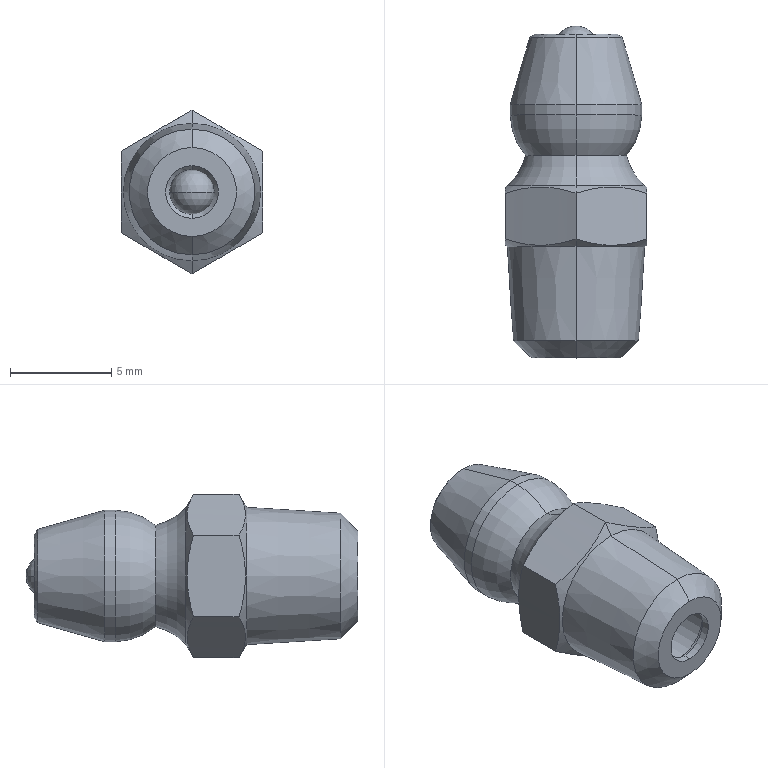Part | SolidWorks | features BaseBody 1 | 1 solid | 40 faces | box 7.001 x 16.4 x 8.083 mm | volume 360.824 mm3 | cone 14 | cylinder 8 | plane 8 | torus 6 | sphere 4 | commonest cylinder face diameters 2 x2 2.6 x2 3.4 x2 6.5 x2
STEP:
#1=CARTESIAN_POINT('',(0.,10.243,-1.007));
#2=VERTEX_POINT('',#1);
#3=CARTESIAN_POINT('',(1.007,10.243,0.));
#4=VERTEX_POINT('',#3);
#5=CARTESIAN_POINT('',(0.,10.243,0.));
#6=DIRECTION('',(0.,-1.,0.));
#7=DIRECTION('',(0.,0.,-1.));
#8=AXIS2_PLACEMENT_3D('',#5,#6,#7);
#9=CIRCLE('',#8,1.007);
#10=EDGE_CURVE('',#2,#4,#9,.T.);
#11=ORIENTED_EDGE('',*,*,#10,.T.);
#12=CARTESIAN_POINT('',(0.,8.7,0.));
#13=VERTEX_POINT('',#12);
#14=CARTESIAN_POINT('',(0.,9.8,0.));
#15=DIRECTION('',(0.,0.,-1.));
#16=DIRECTION('',(-1.,0.,0.));
#17=AXIS2_PLACEMENT_3D('',#14,#15,#16);
#18=CIRCLE('',#17,1.1);
#19=EDGE_CURVE('',#4,#13,#18,.T.);
#20=ORIENTED_EDGE('',*,*,#19,.T.);
#21=CARTESIAN_POINT('',(-1.007,10.243,0.));
#22=VERTEX_POINT('',#21);
#23=CARTESIAN_POINT('',(0.,9.8,0.));
#24=DIRECTION('',(0.,0.,1.));
#25=DIRECTION('',(1.,0.,0.));
#26=AXIS2_PLACEMENT_3D('',#23,#24,#25);
#27=CIRCLE('',#26,1.1);
#28=EDGE_CURVE('',#22,#13,#27,.T.);
#29=ORIENTED_EDGE('',*,*,#28,.F.);
#30=CARTESIAN_POINT('',(0.,10.243,0.));
#31=DIRECTION('',(0.,-1.,0.));
#32=DIRECTION('',(0.,0.,-1.));
#33=AXIS2_PLACEMENT_3D('',#30,#31,#32);
#34=CIRCLE('',#33,1.007);
#35=EDGE_CURVE('',#22,#2,#34,.T.);
#36=ORIENTED_EDGE('',*,*,#35,.T.);
#37=EDGE_LOOP('',(#11,#20,#29,#36));
#38=FACE_OUTER_BOUND('',#37,.T.);
#39=CARTESIAN_POINT('',(0.,9.8,0.));
#40=DIRECTION('',(0.,0.,-1.));
#41=DIRECTION('',(-1.,0.,0.));
#42=AXIS2_PLACEMENT_3D('',#39,#40,#41);
#43=SPHERICAL_SURFACE('',#42,1.1);
#44=ADVANCED_FACE('',(#38),#43,.T.);
#45=CARTESIAN_POINT('',(0.,10.243,1.007));
#46=VERTEX_POINT('',#45);
#47=CARTESIAN_POINT('',(0.,10.243,0.));
#48=DIRECTION('',(0.,-1.,0.));
#49=DIRECTION('',(0.,0.,-1.));
#50=AXIS2_PLACEMENT_3D('',#47,#48,#49);
#51=CIRCLE('',#50,1.007);
#52=EDGE_CURVE('',#46,#22,#51,.T.);
#53=ORIENTED_EDGE('',*,*,#52,.F.);
#54=CARTESIAN_POINT('',(0.,9.55,1.7));
#55=VERTEX_POINT('',#54);
#56=CARTESIAN_POINT('',(0.,9.55,1.7));
#57=DIRECTION('',(0.,-0.7071,0.7071));
#58=VECTOR('',#57,1000.);
#59=LINE('',#56,#58);
#60=EDGE_CURVE('',#46,#55,#59,.T.);
#61=ORIENTED_EDGE('',*,*,#60,.T.);
#62=CARTESIAN_POINT('',(0.,9.55,-1.7));
#63=VERTEX_POINT('',#62);
#64=CARTESIAN_POINT('',(0.,9.55,0.));
#65=DIRECTION('',(0.,-1.,0.));
#66=DIRECTION('',(0.,0.,-1.));
#67=AXIS2_PLACEMENT_3D('',#64,#65,#66);
#68=CIRCLE('',#67,1.7);
#69=EDGE_CURVE('',#55,#63,#68,.T.);
#70=ORIENTED_EDGE('',*,*,#69,.T.);
#71=CARTESIAN_POINT('',(0.,9.55,-1.7));
#72=DIRECTION('',(0.,-0.7071,-0.7071));
#73=VECTOR('',#72,1000.);
#74=LINE('',#71,#73);
#75=EDGE_CURVE('',#2,#63,#74,.T.);
#76=ORIENTED_EDGE('',*,*,#75,.F.);
#77=ORIENTED_EDGE('',*,*,#35,.F.);
#78=EDGE_LOOP('',(#53,#61,#70,#76,#77));
#79=FACE_OUTER_BOUND('',#78,.T.);
#80=CARTESIAN_POINT('',(0.,9.55,0.));
#81=DIRECTION('',(0.,-1.,0.));
#82=DIRECTION('',(0.,0.,-1.));
#83=AXIS2_PLACEMENT_3D('',#80,#81,#82);
#84=CONICAL_SURFACE('',#83,1.7,0.7854);
#85=ADVANCED_FACE('',(#79),#84,.F.);
#86=ORIENTED_EDGE('',*,*,#69,.F.);
#87=CARTESIAN_POINT('',(0.,-4.7,1.7));
#88=VERTEX_POINT('',#87);
#89=CARTESIAN_POINT('',(0.,-5.5,1.7));
#90=DIRECTION('',(0.,-1.,0.));
#91=VECTOR('',#90,1000.);
#92=LINE('',#89,#91);
#93=EDGE_CURVE('',#55,#88,#92,.T.);
#94=ORIENTED_EDGE('',*,*,#93,.T.);
#95=CARTESIAN_POINT('',(0.,-4.7,-1.7));
#96=VERTEX_POINT('',#95);
#97=CARTESIAN_POINT('',(0.,-4.7,0.));
#98=DIRECTION('',(0.,-1.,0.));
#99=DIRECTION('',(0.,0.,-1.));
#100=AXIS2_PLACEMENT_3D('',#97,#98,#99);
#101=CIRCLE('',#100,1.7);
#102=EDGE_CURVE('',#88,#96,#101,.T.);
#103=ORIENTED_EDGE('',*,*,#102,.T.);
#104=CARTESIAN_POINT('',(0.,-5.5,-1.7));
#105=DIRECTION('',(0.,-1.,0.));
#106=VECTOR('',#105,1000.);
#107=LINE('',#104,#106);
#108=EDGE_CURVE('',#63,#96,#107,.T.);
#109=ORIENTED_EDGE('',*,*,#108,.F.);
#110=EDGE_LOOP('',(#86,#94,#103,#109));
#111=FACE_OUTER_BOUND('',#110,.T.);
#112=CARTESIAN_POINT('',(0.,-5.5,0.));
#113=DIRECTION('',(0.,-1.,0.));
#114=DIRECTION('',(0.,0.,-1.));
#115=AXIS2_PLACEMENT_3D('',#112,#113,#114);
#116=CYLINDRICAL_SURFACE('',#115,1.7);
#117=ADVANCED_FACE('',(#111),#116,.F.);
#118=ORIENTED_EDGE('',*,*,#102,.F.);
#119=CARTESIAN_POINT('',(0.,-5.1,1.3));
#120=VERTEX_POINT('',#119);
#121=CARTESIAN_POINT('',(0.,-4.7,1.3));
#122=DIRECTION('',(1.,0.,0.));
#123=DIRECTION('',(0.,0.,-1.));
#124=AXIS2_PLACEMENT_3D('',#121,#122,#123);
#125=CIRCLE('',#124,0.4);
#126=EDGE_CURVE('',#88,#120,#125,.T.);
#127=ORIENTED_EDGE('',*,*,#126,.T.);
#128=CARTESIAN_POINT('',(0.,-5.1,-1.3));
#129=VERTEX_POINT('',#128);
#130=CARTESIAN_POINT('',(0.,-5.1,0.));
#131=DIRECTION('',(0.,-1.,0.));
#132=DIRECTION('',(0.,0.,-1.));
#133=AXIS2_PLACEMENT_3D('',#130,#131,#132);
#134=CIRCLE('',#133,1.3);
#135=EDGE_CURVE('',#120,#129,#134,.T.);
#136=ORIENTED_EDGE('',*,*,#135,.T.);
#137=CARTESIAN_POINT('',(0.,-4.7,-1.3));
#138=DIRECTION('',(-1.,0.,0.));
#139=DIRECTION('',(0.,0.,1.));
#140=AXIS2_PLACEMENT_3D('',#137,#138,#139);
#141=CIRCLE('',#140,0.4);
#142=EDGE_CURVE('',#96,#129,#141,.T.);
#143=ORIENTED_EDGE('',*,*,#142,.F.);
#144=EDGE_LOOP('',(#118,#127,#136,#143));
#145=FACE_OUTER_BOUND('',#144,.T.);
#146=CARTESIAN_POINT('',(0.,-4.7,0.));
#147=DIRECTION('',(0.,-1.,0.));
#148=DIRECTION('',(0.,0.,-1.));
#149=AXIS2_PLACEMENT_3D('',#146,#147,#148);
#150=TOROIDAL_SURFACE('',#149,1.3,0.4);
#151=ADVANCED_FACE('',(#145),#150,.F.);
#152=ORIENTED_EDGE('',*,*,#135,.F.);
#153=CARTESIAN_POINT('',(0.,-5.5,1.3));
#154=VERTEX_POINT('',#153);
#155=CARTESIAN_POINT('',(0.,-5.5,1.3));
#156=DIRECTION('',(0.,-1.,0.));
#157=VECTOR('',#156,1000.);
#158=LINE('',#155,#157);
#159=EDGE_CURVE('',#120,#154,#158,.T.);
#160=ORIENTED_EDGE('',*,*,#159,.T.);
#161=CARTESIAN_POINT('',(0.,-5.5,-1.3));
#162=VERTEX_POINT('',#161);
#163=CARTESIAN_POINT('',(0.,-5.5,0.));
#164=DIRECTION('',(0.,-1.,0.));
#165=DIRECTION('',(0.,0.,-1.));
#166=AXIS2_PLACEMENT_3D('',#163,#164,#165);
#167=CIRCLE('',#166,1.3);
#168=EDGE_CURVE('',#154,#162,#167,.T.);
#169=ORIENTED_EDGE('',*,*,#168,.T.);
#170=CARTESIAN_POINT('',(0.,-5.5,-1.3));
#171=DIRECTION('',(0.,-1.,0.));
#172=VECTOR('',#171,1000.);
#173=LINE('',#170,#172);
#174=EDGE_CURVE('',#129,#162,#173,.T.);
#175=ORIENTED_EDGE('',*,*,#174,.F.);
#176=EDGE_LOOP('',(#152,#160,#169,#175));
#177=FACE_OUTER_BOUND('',#176,.T.);
#178=CARTESIAN_POINT('',(0.,-5.5,0.));
#179=DIRECTION('',(0.,-1.,0.));
#180=DIRECTION('',(0.,0.,-1.));
#181=AXIS2_PLACEMENT_3D('',#178,#179,#180);
#182=CYLINDRICAL_SURFACE('',#181,1.3);
#183=ADVANCED_FACE('',(#177),#182,.F.);
#184=CARTESIAN_POINT('',(0.,-5.5,-2.2));
#185=VERTEX_POINT('',#184);
#186=CARTESIAN_POINT('',(0.,-5.5,2.2));
#187=VERTEX_POINT('',#186);
#188=CARTESIAN_POINT('',(0.,-5.5,0.));
#189=DIRECTION('',(0.,-1.,0.));
#190=DIRECTION('',(0.,0.,-1.));
#191=AXIS2_PLACEMENT_3D('',#188,#189,#190);
#192=CIRCLE('',#191,2.2);
#193=EDGE_CURVE('',#185,#187,#192,.T.);
#194=ORIENTED_EDGE('',*,*,#193,.F.);
#195=CARTESIAN_POINT('',(0.,-4.652,-3.103));
#196=VERTEX_POINT('',#195);
#197=CARTESIAN_POINT('',(0.,-4.652,-3.103));
#198=DIRECTION('',(0.,0.6847,-0.7288));
#199=VECTOR('',#198,1000.);
#200=LINE('',#197,#199);
#201=EDGE_CURVE('',#185,#196,#200,.T.);
#202=ORIENTED_EDGE('',*,*,#201,.T.);
#203=CARTESIAN_POINT('',(0.,-4.652,3.103));
#204=VERTEX_POINT('',#203);
#205=CARTESIAN_POINT('',(0.,-4.652,0.));
#206=DIRECTION('',(0.,-1.,0.));
#207=DIRECTION('',(0.,0.,-1.));
#208=AXIS2_PLACEMENT_3D('',#205,#206,#207);
#209=CIRCLE('',#208,3.103);
#210=EDGE_CURVE('',#196,#204,#209,.T.);
#211=ORIENTED_EDGE('',*,*,#210,.T.);
#212=CARTESIAN_POINT('',(0.,-4.652,3.103));
#213=DIRECTION('',(0.,0.6847,0.7288));
#214=VECTOR('',#213,1000.);
#215=LINE('',#212,#214);
#216=EDGE_CURVE('',#187,#204,#215,.T.);
#217=ORIENTED_EDGE('',*,*,#216,.F.);
#218=EDGE_LOOP('',(#194,#202,#211,#217));
#219=FACE_OUTER_BOUND('',#218,.T.);
#220=CARTESIAN_POINT('',(0.,-4.652,0.));
#221=DIRECTION('',(0.,1.,0.));
#222=DIRECTION('',(0.,0.,1.));
#223=AXIS2_PLACEMENT_3D('',#220,#221,#222);
#224=CONICAL_SURFACE('',#223,3.103,0.8166);
#225=ADVANCED_FACE('',(#219),#224,.T.);
#226=ORIENTED_EDGE('',*,*,#210,.F.);
#227=CARTESIAN_POINT('',(0.,0.,-3.394));
#228=VERTEX_POINT('',#227);
#229=CARTESIAN_POINT('',(0.,0.,-3.394));
#230=DIRECTION('',(0.,0.998,-0.06244));
#231=VECTOR('',#230,1000.);
#232=LINE('',#229,#231);
#233=EDGE_CURVE('',#196,#228,#232,.T.);
#234=ORIENTED_EDGE('',*,*,#233,.T.);
#235=CARTESIAN_POINT('',(0.,0.,3.394));
#236=VERTEX_POINT('',#235);
#237=CARTESIAN_POINT('',(0.,0.,0.));
#238=DIRECTION('',(0.,-1.,0.));
#239=DIRECTION('',(0.,0.,-1.));
#240=AXIS2_PLACEMENT_3D('',#237,#238,#239);
#241=CIRCLE('',#240,3.394);
#242=EDGE_CURVE('',#228,#236,#241,.T.);
#243=ORIENTED_EDGE('',*,*,#242,.T.);
#244=CARTESIAN_POINT('',(0.,0.,3.394));
#245=DIRECTION('',(0.,0.998,0.06244));
#246=VECTOR('',#245,1000.);
#247=LINE('',#244,#246);
#248=EDGE_CURVE('',#204,#236,#247,.T.);
#249=ORIENTED_EDGE('',*,*,#248,.F.);
#250=EDGE_LOOP('',(#226,#234,#243,#249));
#251=FACE_OUTER_BOUND('',#250,.T.);
#252=CARTESIAN_POINT('',(0.,0.,0.));
#253=DIRECTION('',(0.,1.,0.));
#254=DIRECTION('',(0.,0.,1.));
#255=AXIS2_PLACEMENT_3D('',#252,#253,#254);
#256=CONICAL_SURFACE('',#255,3.394,0.06248);
#257=ADVANCED_FACE('',(#251),#256,.T.);
#258=ORIENTED_EDGE('',*,*,#242,.F.);
#259=CARTESIAN_POINT('',(0.,0.374,-4.041));
#260=VERTEX_POINT('',#259);
#261=CARTESIAN_POINT('',(0.,1.216,-5.5));
#262=DIRECTION('',(0.,0.5,-0.866));
#263=VECTOR('',#262,1000.);
#264=LINE('',#261,#263);
#265=EDGE_CURVE('',#228,#260,#264,.T.);
#266=ORIENTED_EDGE('',*,*,#265,.T.);
#267=CARTESIAN_POINT('',(3.5,0.374,-2.021));
#268=VERTEX_POINT('',#267);
#269=CARTESIAN_POINT('',(0.,0.374,-4.041));
#270=CARTESIAN_POINT('',(0.1588,0.321,-3.95));
#271=CARTESIAN_POINT('',(0.303,0.2771,-3.865));
#272=CARTESIAN_POINT('',(0.585,0.2025,-3.702));
#273=CARTESIAN_POINT('',(0.7229,0.1719,-3.623));
#274=CARTESIAN_POINT('',(1.15,0.09295,-3.378));
#275=CARTESIAN_POINT('',(1.457,0.0621,-3.201));
#276=CARTESIAN_POINT('',(1.896,0.0612,-2.946));
#277=CARTESIAN_POINT('',(2.041,0.0685,-2.864));
#278=CARTESIAN_POINT('',(2.338,0.09717,-2.693));
#279=CARTESIAN_POINT('',(2.488,0.1184,-2.606));
#280=CARTESIAN_POINT('',(2.78,0.1726,-2.436));
#281=CARTESIAN_POINT('',(2.918,0.2041,-2.355));
#282=CARTESIAN_POINT('',(3.199,0.2783,-2.193));
#283=CARTESIAN_POINT('',(3.343,0.3216,-2.111));
#284=CARTESIAN_POINT('',(3.5,0.374,-2.021));
#285=B_SPLINE_CURVE_WITH_KNOTS('',3,(#269,#270,#271,#272,#273,#274,#275,#276,#277,#278,#279,#280,#281,#282,#283,#284),.UNSPECIFIED.,.F.,.F.,(4,2,2,2,2,2,2,4),(0.0002381,0.5104,1.021,2.041,2.551,3.061,3.572,4.082),.UNSPECIFIED.);
#286=EDGE_CURVE('',#260,#268,#285,.T.);
#287=ORIENTED_EDGE('',*,*,#286,.T.);
#288=CARTESIAN_POINT('',(3.5,0.374,2.021));
#289=VERTEX_POINT('',#288);
#290=CARTESIAN_POINT('',(3.5,0.374,-2.021));
#291=CARTESIAN_POINT('',(3.5,0.3259,-1.854));
#292=CARTESIAN_POINT('',(3.5,0.2835,-1.693));
#293=CARTESIAN_POINT('',(3.5,0.2061,-1.357));
#294=CARTESIAN_POINT('',(3.5,0.1735,-1.194));
#295=CARTESIAN_POINT('',(3.5,0.1183,-0.8526));
#296=CARTESIAN_POINT('',(3.501,0.09717,-0.6799));
#297=CARTESIAN_POINT('',(3.501,0.06865,-0.337));
#298=CARTESIAN_POINT('',(3.5,0.06131,-0.1677));
#299=CARTESIAN_POINT('',(3.5,0.06147,0.3344));
#300=CARTESIAN_POINT('',(3.5,0.09108,0.6846));
#301=CARTESIAN_POINT('',(3.5,0.1735,1.194));
#302=CARTESIAN_POINT('',(3.5,0.2062,1.357));
#303=CARTESIAN_POINT('',(3.5,0.2835,1.693));
#304=CARTESIAN_POINT('',(3.5,0.3263,1.856));
#305=CARTESIAN_POINT('',(3.5,0.374,2.021));
#306=B_SPLINE_CURVE_WITH_KNOTS('',3,(#290,#291,#292,#293,#294,#295,#296,#297,#298,#299,#300,#301,#302,#303,#304,#305),.UNSPECIFIED.,.F.,.F.,(4,2,2,2,2,2,2,4),(4.59,5.104,5.618,6.132,6.646,7.674,8.188,8.702),.UNSPECIFIED.);
#307=EDGE_CURVE('',#268,#289,#306,.T.);
#308=ORIENTED_EDGE('',*,*,#307,.T.);
#309=CARTESIAN_POINT('',(0.,0.374,4.041));
#310=VERTEX_POINT('',#309);
#311=CARTESIAN_POINT('',(3.5,0.374,2.021));
#312=CARTESIAN_POINT('',(3.341,0.321,2.112));
#313=CARTESIAN_POINT('',(3.195,0.2771,2.195));
#314=CARTESIAN_POINT('',(2.913,0.2025,2.357));
#315=CARTESIAN_POINT('',(2.777,0.1719,2.438));
#316=CARTESIAN_POINT('',(2.35,0.09295,2.685));
#317=CARTESIAN_POINT('',(2.044,0.0621,2.863));
#318=CARTESIAN_POINT('',(1.604,0.0612,3.115));
#319=CARTESIAN_POINT('',(1.46,0.0685,3.199));
#320=CARTESIAN_POINT('',(1.163,0.09717,3.371));
#321=CARTESIAN_POINT('',(1.013,0.1184,3.457));
#322=CARTESIAN_POINT('',(0.7202,0.1726,3.625));
#323=CARTESIAN_POINT('',(0.5806,0.2041,3.705));
#324=CARTESIAN_POINT('',(0.2992,0.2783,3.867));
#325=CARTESIAN_POINT('',(0.1571,0.3216,3.951));
#326=CARTESIAN_POINT('',(0.,0.374,4.041));
#327=B_SPLINE_CURVE_WITH_KNOTS('',3,(#311,#312,#313,#314,#315,#316,#317,#318,#319,#320,#321,#322,#323,#324,#325,#326),.UNSPECIFIED.,.F.,.F.,(4,2,2,2,2,2,2,4),(0.0002381,0.5104,1.021,2.041,2.551,3.061,3.572,4.082),.UNSPECIFIED.);
#328=EDGE_CURVE('',#289,#310,#327,.T.);
#329=ORIENTED_EDGE('',*,*,#328,.T.);
#330=CARTESIAN_POINT('',(0.,1.216,5.5));
#331=DIRECTION('',(0.,0.5,0.866));
#332=VECTOR('',#331,1000.);
#333=LINE('',#330,#332);
#334=EDGE_CURVE('',#236,#310,#333,.T.);
#335=ORIENTED_EDGE('',*,*,#334,.F.);
#336=EDGE_LOOP('',(#258,#266,#287,#308,#329,#335));
#337=FACE_OUTER_BOUND('',#336,.T.);
#338=CARTESIAN_POINT('',(0.,1.216,0.));
#339=DIRECTION('',(0.,1.,0.));
#340=DIRECTION('',(0.,0.,1.));
#341=AXIS2_PLACEMENT_3D('',#338,#339,#340);
#342=CONICAL_SURFACE('',#341,5.5,1.047);
#343=ADVANCED_FACE('',(#337),#342,.T.);
#344=CARTESIAN_POINT('',(0.,3.,-3.394));
#345=VERTEX_POINT('',#344);
#346=CARTESIAN_POINT('',(0.,3.,3.394));
#347=VERTEX_POINT('',#346);
#348=CARTESIAN_POINT('',(0.,3.,0.));
#349=DIRECTION('',(0.,-1.,0.));
#350=DIRECTION('',(0.,0.,-1.));
#351=AXIS2_PLACEMENT_3D('',#348,#349,#350);
#352=CIRCLE('',#351,3.394);
#353=EDGE_CURVE('',#345,#347,#352,.T.);
#354=ORIENTED_EDGE('',*,*,#353,.T.);
#355=CARTESIAN_POINT('',(0.,2.626,4.041));
#356=VERTEX_POINT('',#355);
#357=CARTESIAN_POINT('',(0.,3.,3.394));
#358=DIRECTION('',(0.,-0.5,0.866));
#359=VECTOR('',#358,1000.);
#360=LINE('',#357,#359);
#361=EDGE_CURVE('',#347,#356,#360,.T.);
#362=ORIENTED_EDGE('',*,*,#361,.T.);
#363=CARTESIAN_POINT('',(3.5,2.626,2.021));
#364=VERTEX_POINT('',#363);
#365=CARTESIAN_POINT('',(0.,2.626,4.041));
#366=CARTESIAN_POINT('',(0.1588,2.679,3.95));
#367=CARTESIAN_POINT('',(0.303,2.723,3.865));
#368=CARTESIAN_POINT('',(0.585,2.797,3.702));
#369=CARTESIAN_POINT('',(0.7229,2.828,3.623));
#370=CARTESIAN_POINT('',(1.15,2.907,3.378));
#371=CARTESIAN_POINT('',(1.457,2.938,3.201));
#372=CARTESIAN_POINT('',(1.896,2.939,2.946));
#373=CARTESIAN_POINT('',(2.041,2.932,2.864));
#374=CARTESIAN_POINT('',(2.338,2.903,2.693));
#375=CARTESIAN_POINT('',(2.488,2.882,2.606));
#376=CARTESIAN_POINT('',(2.78,2.827,2.436));
#377=CARTESIAN_POINT('',(2.918,2.796,2.355));
#378=CARTESIAN_POINT('',(3.199,2.722,2.193));
#379=CARTESIAN_POINT('',(3.343,2.678,2.111));
#380=CARTESIAN_POINT('',(3.5,2.626,2.021));
#381=B_SPLINE_CURVE_WITH_KNOTS('',3,(#365,#366,#367,#368,#369,#370,#371,#372,#373,#374,#375,#376,#377,#378,#379,#380),.UNSPECIFIED.,.F.,.F.,(4,2,2,2,2,2,2,4),(0.0002381,0.5104,1.021,2.041,2.551,3.061,3.572,4.082),.UNSPECIFIED.);
#382=EDGE_CURVE('',#356,#364,#381,.T.);
#383=ORIENTED_EDGE('',*,*,#382,.T.);
#384=CARTESIAN_POINT('',(3.5,2.626,-2.021));
#385=VERTEX_POINT('',#384);
#386=CARTESIAN_POINT('',(3.5,2.626,2.021));
#387=CARTESIAN_POINT('',(3.5,2.674,1.854));
#388=CARTESIAN_POINT('',(3.5,2.716,1.693));
#389=CARTESIAN_POINT('',(3.5,2.794,1.357));
#390=CARTESIAN_POINT('',(3.5,2.826,1.194));
#391=CARTESIAN_POINT('',(3.5,2.882,0.8526));
#392=CARTESIAN_POINT('',(3.501,2.903,0.6799));
#393=CARTESIAN_POINT('',(3.501,2.931,0.337));
#394=CARTESIAN_POINT('',(3.5,2.939,0.1677));
#395=CARTESIAN_POINT('',(3.5,2.939,-0.3344));
#396=CARTESIAN_POINT('',(3.5,2.909,-0.6846));
#397=CARTESIAN_POINT('',(3.5,2.826,-1.194));
#398=CARTESIAN_POINT('',(3.5,2.794,-1.357));
#399=CARTESIAN_POINT('',(3.5,2.716,-1.693));
#400=CARTESIAN_POINT('',(3.5,2.674,-1.856));
#401=CARTESIAN_POINT('',(3.5,2.626,-2.021));
#402=B_SPLINE_CURVE_WITH_KNOTS('',3,(#386,#387,#388,#389,#390,#391,#392,#393,#394,#395,#396,#397,#398,#399,#400,#401),.UNSPECIFIED.,.F.,.F.,(4,2,2,2,2,2,2,4),(4.59,5.104,5.618,6.132,6.646,7.674,8.188,8.702),.UNSPECIFIED.);
#403=EDGE_CURVE('',#364,#385,#402,.T.);
#404=ORIENTED_EDGE('',*,*,#403,.T.);
#405=CARTESIAN_POINT('',(0.,2.626,-4.041));
#406=VERTEX_POINT('',#405);
#407=CARTESIAN_POINT('',(3.5,2.626,-2.021));
#408=CARTESIAN_POINT('',(3.341,2.679,-2.112));
#409=CARTESIAN_POINT('',(3.195,2.723,-2.195));
#410=CARTESIAN_POINT('',(2.913,2.797,-2.357));
#411=CARTESIAN_POINT('',(2.777,2.828,-2.438));
#412=CARTESIAN_POINT('',(2.35,2.907,-2.685));
#413=CARTESIAN_POINT('',(2.044,2.938,-2.863));
#414=CARTESIAN_POINT('',(1.604,2.939,-3.115));
#415=CARTESIAN_POINT('',(1.46,2.932,-3.199));
#416=CARTESIAN_POINT('',(1.163,2.903,-3.371));
#417=CARTESIAN_POINT('',(1.013,2.882,-3.457));
#418=CARTESIAN_POINT('',(0.7202,2.827,-3.625));
#419=CARTESIAN_POINT('',(0.5806,2.796,-3.705));
#420=CARTESIAN_POINT('',(0.2992,2.722,-3.867));
#421=CARTESIAN_POINT('',(0.1571,2.678,-3.951));
#422=CARTESIAN_POINT('',(0.,2.626,-4.041));
#423=B_SPLINE_CURVE_WITH_KNOTS('',3,(#407,#408,#409,#410,#411,#412,#413,#414,#415,#416,#417,#418,#419,#420,#421,#422),.UNSPECIFIED.,.F.,.F.,(4,2,2,2,2,2,2,4),(0.0002381,0.5104,1.021,2.041,2.551,3.061,3.572,4.082),.UNSPECIFIED.);
#424=EDGE_CURVE('',#385,#406,#423,.T.);
#425=ORIENTED_EDGE('',*,*,#424,.T.);
#426=CARTESIAN_POINT('',(0.,3.,-3.394));
#427=DIRECTION('',(0.,-0.5,-0.866));
#428=VECTOR('',#427,1000.);
#429=LINE('',#426,#428);
#430=EDGE_CURVE('',#345,#406,#429,.T.);
#431=ORIENTED_EDGE('',*,*,#430,.F.);
#432=EDGE_LOOP('',(#354,#362,#383,#404,#425,#431));
#433=FACE_OUTER_BOUND('',#432,.T.);
#434=CARTESIAN_POINT('',(0.,3.,0.));
#435=DIRECTION('',(0.,-1.,0.));
#436=DIRECTION('',(0.,0.,-1.));
#437=AXIS2_PLACEMENT_3D('',#434,#435,#436);
#438=CONICAL_SURFACE('',#437,3.394,1.047);
#439=ADVANCED_FACE('',(#433),#438,.T.);
#440=CARTESIAN_POINT('',(0.,3.,0.));
#441=DIRECTION('',(0.,-1.,0.));
#442=DIRECTION('',(0.,0.,-1.));
#443=AXIS2_PLACEMENT_3D('',#440,#441,#442);
#444=CIRCLE('',#443,3.394);
#445=EDGE_CURVE('',#347,#345,#444,.T.);
#446=ORIENTED_EDGE('',*,*,#445,.F.);
#447=CARTESIAN_POINT('',(0.,4.5,2.5));
#448=VERTEX_POINT('',#447);
#449=CARTESIAN_POINT('',(0.,5.166,5.323));
#450=DIRECTION('',(1.,0.,0.));
#451=DIRECTION('',(0.,0.,-1.));
#452=AXIS2_PLACEMENT_3D('',#449,#450,#451);
#453=CIRCLE('',#452,2.9);
#454=EDGE_CURVE('',#347,#448,#453,.T.);
#455=ORIENTED_EDGE('',*,*,#454,.T.);
#456=CARTESIAN_POINT('',(0.,4.5,-2.5));
#457=VERTEX_POINT('',#456);
#458=CARTESIAN_POINT('',(0.,4.5,0.));
#459=DIRECTION('',(0.,-1.,0.));
#460=DIRECTION('',(0.,0.,-1.));
#461=AXIS2_PLACEMENT_3D('',#458,#459,#460);
#462=CIRCLE('',#461,2.5);
#463=EDGE_CURVE('',#448,#457,#462,.T.);
#464=ORIENTED_EDGE('',*,*,#463,.T.);
#465=CARTESIAN_POINT('',(0.,5.166,-5.323));
#466=DIRECTION('',(-1.,0.,0.));
#467=DIRECTION('',(0.,0.,1.));
#468=AXIS2_PLACEMENT_3D('',#465,#466,#467);
#469=CIRCLE('',#468,2.9);
#470=EDGE_CURVE('',#345,#457,#469,.T.);
#471=ORIENTED_EDGE('',*,*,#470,.F.);
#472=EDGE_LOOP('',(#446,#455,#464,#471));
#473=FACE_OUTER_BOUND('',#472,.T.);
#474=CARTESIAN_POINT('',(0.,5.166,0.));
#475=DIRECTION('',(0.,-1.,0.));
#476=DIRECTION('',(0.,0.,-1.));
#477=AXIS2_PLACEMENT_3D('',#474,#475,#476);
#478=TOROIDAL_SURFACE('',#477,5.323,2.9);
#479=ADVANCED_FACE('',(#473),#478,.F.);
#480=CARTESIAN_POINT('',(0.,6.5,-3.25));
#481=VERTEX_POINT('',#480);
#482=CARTESIAN_POINT('',(0.,6.5,3.25));
#483=VERTEX_POINT('',#482);
#484=CARTESIAN_POINT('',(0.,6.5,0.));
#485=DIRECTION('',(0.,-1.,0.));
#486=DIRECTION('',(0.,0.,-1.));
#487=AXIS2_PLACEMENT_3D('',#484,#485,#486);
#488=CIRCLE('',#487,3.25);
#489=EDGE_CURVE('',#481,#483,#488,.T.);
#490=ORIENTED_EDGE('',*,*,#489,.T.);
#491=CARTESIAN_POINT('',(0.,6.578,0.0009308));
#492=DIRECTION('',(1.,0.,0.));
#493=DIRECTION('',(0.,0.,-1.));
#494=AXIS2_PLACEMENT_3D('',#491,#492,#493);
#495=CIRCLE('',#494,3.25);
#496=EDGE_CURVE('',#483,#448,#495,.T.);
#497=ORIENTED_EDGE('',*,*,#496,.T.);
#498=CARTESIAN_POINT('',(0.,4.5,0.));
#499=DIRECTION('',(0.,-1.,0.));
#500=DIRECTION('',(0.,0.,-1.));
#501=AXIS2_PLACEMENT_3D('',#498,#499,#500);
#502=CIRCLE('',#501,2.5);
#503=EDGE_CURVE('',#457,#448,#502,.T.);
#504=ORIENTED_EDGE('',*,*,#503,.F.);
#505=CARTESIAN_POINT('',(0.,6.578,-0.0009308));
#506=DIRECTION('',(-1.,0.,0.));
#507=DIRECTION('',(0.,0.,1.));
#508=AXIS2_PLACEMENT_3D('',#505,#506,#507);
#509=CIRCLE('',#508,3.25);
#510=EDGE_CURVE('',#481,#457,#509,.T.);
#511=ORIENTED_EDGE('',*,*,#510,.F.);
#512=EDGE_LOOP('',(#490,#497,#504,#511));
#513=FACE_OUTER_BOUND('',#512,.T.);
#514=CARTESIAN_POINT('',(0.,6.578,0.));
#515=DIRECTION('',(0.,-1.,0.));
#516=DIRECTION('',(0.,0.,-1.));
#517=AXIS2_PLACEMENT_3D('',#514,#515,#516);
#518=TOROIDAL_SURFACE('',#517,0.0009308,3.25);
#519=ADVANCED_FACE('',(#513),#518,.T.);
#520=CARTESIAN_POINT('',(0.,7.,-3.25));
#521=VERTEX_POINT('',#520);
#522=CARTESIAN_POINT('',(0.,7.,3.25));
#523=VERTEX_POINT('',#522);
#524=CARTESIAN_POINT('',(0.,7.,0.));
#525=DIRECTION('',(0.,-1.,0.));
#526=DIRECTION('',(0.,0.,-1.));
#527=AXIS2_PLACEMENT_3D('',#524,#525,#526);
#528=CIRCLE('',#527,3.25);
#529=EDGE_CURVE('',#521,#523,#528,.T.);
#530=ORIENTED_EDGE('',*,*,#529,.T.);
#531=CARTESIAN_POINT('',(0.,-5.5,3.25));
#532=DIRECTION('',(0.,-1.,0.));
#533=VECTOR('',#532,1000.);
#534=LINE('',#531,#533);
#535=EDGE_CURVE('',#523,#483,#534,.T.);
#536=ORIENTED_EDGE('',*,*,#535,.T.);
#537=ORIENTED_EDGE('',*,*,#489,.F.);
#538=CARTESIAN_POINT('',(0.,-5.5,-3.25));
#539=DIRECTION('',(0.,-1.,0.));
#540=VECTOR('',#539,1000.);
#541=LINE('',#538,#540);
#542=EDGE_CURVE('',#521,#481,#541,.T.);
#543=ORIENTED_EDGE('',*,*,#542,.F.);
#544=EDGE_LOOP('',(#530,#536,#537,#543));
#545=FACE_OUTER_BOUND('',#544,.T.);
#546=CARTESIAN_POINT('',(0.,-5.5,0.));
#547=DIRECTION('',(0.,-1.,0.));
#548=DIRECTION('',(0.,0.,-1.));
#549=AXIS2_PLACEMENT_3D('',#546,#547,#548);
#550=CYLINDRICAL_SURFACE('',#549,3.25);
#551=ADVANCED_FACE('',(#545),#550,.T.);
#552=CARTESIAN_POINT('',(0.,10.315,-2.303));
#553=VERTEX_POINT('',#552);
#554=CARTESIAN_POINT('',(0.,10.315,2.303));
#555=VERTEX_POINT('',#554);
#556=CARTESIAN_POINT('',(0.,10.315,0.));
#557=DIRECTION('',(0.,-1.,0.));
#558=DIRECTION('',(0.,0.,-1.));
#559=AXIS2_PLACEMENT_3D('',#556,#557,#558);
#560=CIRCLE('',#559,2.303);
#561=EDGE_CURVE('',#553,#555,#560,.T.);
#562=ORIENTED_EDGE('',*,*,#561,.T.);
#563=CARTESIAN_POINT('',(0.,10.315,2.303));
#564=DIRECTION('',(0.,-0.9615,0.2748));
#565=VECTOR('',#564,1000.);
#566=LINE('',#563,#565);
#567=EDGE_CURVE('',#555,#523,#566,.T.);
#568=ORIENTED_EDGE('',*,*,#567,.T.);
#569=ORIENTED_EDGE('',*,*,#529,.F.);
#570=CARTESIAN_POINT('',(0.,10.315,-2.303));
#571=DIRECTION('',(0.,-0.9615,-0.2748));
#572=VECTOR('',#571,1000.);
#573=LINE('',#570,#572);
#574=EDGE_CURVE('',#553,#521,#573,.T.);
#575=ORIENTED_EDGE('',*,*,#574,.F.);
#576=EDGE_LOOP('',(#562,#568,#569,#575));
#577=FACE_OUTER_BOUND('',#576,.T.);
#578=CARTESIAN_POINT('',(0.,10.315,0.));
#579=DIRECTION('',(0.,-1.,0.));
#580=DIRECTION('',(0.,0.,-1.));
#581=AXIS2_PLACEMENT_3D('',#578,#579,#580);
#582=CONICAL_SURFACE('',#581,2.303,0.2784);
#583=ADVANCED_FACE('',(#577),#582,.T.);
#584=CARTESIAN_POINT('',(0.,10.5,-2.057));
#585=VERTEX_POINT('',#584);
#586=CARTESIAN_POINT('',(0.,10.5,2.057));
#587=VERTEX_POINT('',#586);
#588=CARTESIAN_POINT('',(0.,10.5,0.));
#589=DIRECTION('',(0.,-1.,0.));
#590=DIRECTION('',(0.,0.,-1.));
#591=AXIS2_PLACEMENT_3D('',#588,#589,#590);
#592=CIRCLE('',#591,2.057);
#593=EDGE_CURVE('',#585,#587,#592,.T.);
#594=ORIENTED_EDGE('',*,*,#593,.T.);
#595=CARTESIAN_POINT('',(0.,10.5,2.057));
#596=DIRECTION('',(0.,-0.6022,0.7984));
#597=VECTOR('',#596,1000.);
#598=LINE('',#595,#597);
#599=EDGE_CURVE('',#587,#555,#598,.T.);
#600=ORIENTED_EDGE('',*,*,#599,.T.);
#601=ORIENTED_EDGE('',*,*,#561,.F.);
#602=CARTESIAN_POINT('',(0.,10.5,-2.057));
#603=DIRECTION('',(0.,-0.6022,-0.7984));
#604=VECTOR('',#603,1000.);
#605=LINE('',#602,#604);
#606=EDGE_CURVE('',#585,#553,#605,.T.);
#607=ORIENTED_EDGE('',*,*,#606,.F.);
#608=EDGE_LOOP('',(#594,#600,#601,#607));
#609=FACE_OUTER_BOUND('',#608,.T.);
#610=CARTESIAN_POINT('',(0.,10.5,0.));
#611=DIRECTION('',(0.,-1.,0.));
#612=DIRECTION('',(0.,0.,-1.));
#613=AXIS2_PLACEMENT_3D('',#610,#611,#612);
#614=CONICAL_SURFACE('',#613,2.057,0.9246);
#615=ADVANCED_FACE('',(#609),#614,.T.);
#616=CARTESIAN_POINT('',(0.,10.5,1.));
#617=VERTEX_POINT('',#616);
#618=CARTESIAN_POINT('',(0.,10.5,-1.));
#619=VERTEX_POINT('',#618);
#620=CARTESIAN_POINT('',(0.,10.5,0.));
#621=DIRECTION('',(0.,-1.,0.));
#622=DIRECTION('',(0.,0.,-1.));
#623=AXIS2_PLACEMENT_3D('',#620,#621,#622);
#624=CIRCLE('',#623,1.);
#625=EDGE_CURVE('',#617,#619,#624,.T.);
#626=ORIENTED_EDGE('',*,*,#625,.F.);
#627=CARTESIAN_POINT('',(0.,10.258,1.));
#628=VERTEX_POINT('',#627);
#629=CARTESIAN_POINT('',(0.,-5.5,1.));
#630=DIRECTION('',(0.,-1.,0.));
#631=VECTOR('',#630,1000.);
#632=LINE('',#629,#631);
#633=EDGE_CURVE('',#617,#628,#632,.T.);
#634=ORIENTED_EDGE('',*,*,#633,.T.);
#635=CARTESIAN_POINT('',(-1.,10.258,0.));
#636=VERTEX_POINT('',#635);
#637=CARTESIAN_POINT('',(0.,10.258,0.));
#638=DIRECTION('',(0.,-1.,0.));
#639=DIRECTION('',(0.,0.,-1.));
#640=AXIS2_PLACEMENT_3D('',#637,#638,#639);
#641=CIRCLE('',#640,1.);
#642=EDGE_CURVE('',#628,#636,#641,.T.);
#643=ORIENTED_EDGE('',*,*,#642,.T.);
#644=CARTESIAN_POINT('',(0.,10.258,-1.));
#645=VERTEX_POINT('',#644);
#646=CARTESIAN_POINT('',(0.,10.258,0.));
#647=DIRECTION('',(0.,-1.,0.));
#648=DIRECTION('',(0.,0.,-1.));
#649=AXIS2_PLACEMENT_3D('',#646,#647,#648);
#650=CIRCLE('',#649,1.);
#651=EDGE_CURVE('',#636,#645,#650,.T.);
#652=ORIENTED_EDGE('',*,*,#651,.T.);
#653=CARTESIAN_POINT('',(0.,-5.5,-1.));
#654=DIRECTION('',(0.,-1.,0.));
#655=VECTOR('',#654,1000.);
#656=LINE('',#653,#655);
#657=EDGE_CURVE('',#619,#645,#656,.T.);
#658=ORIENTED_EDGE('',*,*,#657,.F.);
#659=EDGE_LOOP('',(#626,#634,#643,#652,#658));
#660=FACE_OUTER_BOUND('',#659,.T.);
#661=CARTESIAN_POINT('',(0.,-5.5,0.));
#662=DIRECTION('',(0.,-1.,0.));
#663=DIRECTION('',(0.,0.,-1.));
#664=AXIS2_PLACEMENT_3D('',#661,#662,#663);
#665=CYLINDRICAL_SURFACE('',#664,1.);
#666=ADVANCED_FACE('',(#660),#665,.F.);
#667=CARTESIAN_POINT('',(0.,10.9,0.));
#668=VERTEX_POINT('',#667);
#669=CARTESIAN_POINT('',(1.,10.258,0.));
#670=VERTEX_POINT('',#669);
#671=CARTESIAN_POINT('',(0.,9.8,0.));
#672=DIRECTION('',(0.,0.,-1.));
#673=DIRECTION('',(-1.,0.,0.));
#674=AXIS2_PLACEMENT_3D('',#671,#672,#673);
#675=CIRCLE('',#674,1.1);
#676=EDGE_CURVE('',#668,#670,#675,.T.);
#677=ORIENTED_EDGE('',*,*,#676,.F.);
#678=CARTESIAN_POINT('',(0.,9.8,0.));
#679=DIRECTION('',(0.,0.,1.));
#680=DIRECTION('',(1.,0.,0.));
#681=AXIS2_PLACEMENT_3D('',#678,#679,#680);
#682=CIRCLE('',#681,1.1);
#683=EDGE_CURVE('',#668,#636,#682,.T.);
#684=ORIENTED_EDGE('',*,*,#683,.T.);
#685=ORIENTED_EDGE('',*,*,#642,.F.);
#686=CARTESIAN_POINT('',(0.,10.258,0.));
#687=DIRECTION('',(0.,-1.,0.));
#688=DIRECTION('',(0.,0.,-1.));
#689=AXIS2_PLACEMENT_3D('',#686,#687,#688);
#690=CIRCLE('',#689,1.);
#691=EDGE_CURVE('',#670,#628,#690,.T.);
#692=ORIENTED_EDGE('',*,*,#691,.F.);
#693=EDGE_LOOP('',(#677,#684,#685,#692));
#694=FACE_OUTER_BOUND('',#693,.T.);
#695=CARTESIAN_POINT('',(0.,9.8,0.));
#696=DIRECTION('',(0.,0.,1.));
#697=DIRECTION('',(1.,0.,0.));
#698=AXIS2_PLACEMENT_3D('',#695,#696,#697);
#699=SPHERICAL_SURFACE('',#698,1.1);
#700=ADVANCED_FACE('',(#694),#699,.T.);
#701=ORIENTED_EDGE('',*,*,#683,.F.);
#702=ORIENTED_EDGE('',*,*,#676,.T.);
#703=CARTESIAN_POINT('',(0.,10.258,0.));
#704=DIRECTION('',(0.,-1.,0.));
#705=DIRECTION('',(0.,0.,-1.));
#706=AXIS2_PLACEMENT_3D('',#703,#704,#705);
#707=CIRCLE('',#706,1.);
#708=EDGE_CURVE('',#645,#670,#707,.T.);
#709=ORIENTED_EDGE('',*,*,#708,.F.);
#710=ORIENTED_EDGE('',*,*,#651,.F.);
#711=EDGE_LOOP('',(#701,#702,#709,#710));
#712=FACE_OUTER_BOUND('',#711,.T.);
#713=CARTESIAN_POINT('',(0.,9.8,0.));
#714=DIRECTION('',(0.,0.,1.));
#715=DIRECTION('',(1.,0.,0.));
#716=AXIS2_PLACEMENT_3D('',#713,#714,#715);
#717=SPHERICAL_SURFACE('',#716,1.1);
#718=ADVANCED_FACE('',(#712),#717,.T.);
#719=ORIENTED_EDGE('',*,*,#633,.F.);
#720=CARTESIAN_POINT('',(0.,10.5,0.));
#721=DIRECTION('',(0.,-1.,0.));
#722=DIRECTION('',(0.,0.,-1.));
#723=AXIS2_PLACEMENT_3D('',#720,#721,#722);
#724=CIRCLE('',#723,1.);
#725=EDGE_CURVE('',#619,#617,#724,.T.);
#726=ORIENTED_EDGE('',*,*,#725,.F.);
#727=ORIENTED_EDGE('',*,*,#657,.T.);
#728=ORIENTED_EDGE('',*,*,#708,.T.);
#729=ORIENTED_EDGE('',*,*,#691,.T.);
#730=EDGE_LOOP('',(#719,#726,#727,#728,#729));
#731=FACE_OUTER_BOUND('',#730,.T.);
#732=CARTESIAN_POINT('',(0.,-5.5,0.));
#733=DIRECTION('',(0.,-1.,0.));
#734=DIRECTION('',(0.,0.,-1.));
#735=AXIS2_PLACEMENT_3D('',#732,#733,#734);
#736=CYLINDRICAL_SURFACE('',#735,1.);
#737=ADVANCED_FACE('',(#731),#736,.F.);
#738=ORIENTED_EDGE('',*,*,#593,.F.);
#739=CARTESIAN_POINT('',(0.,10.5,0.));
#740=DIRECTION('',(0.,-1.,0.));
#741=DIRECTION('',(0.,0.,-1.));
#742=AXIS2_PLACEMENT_3D('',#739,#740,#741);
#743=CIRCLE('',#742,2.057);
#744=EDGE_CURVE('',#587,#585,#743,.T.);
#745=ORIENTED_EDGE('',*,*,#744,.F.);
#746=EDGE_LOOP('',(#738,#745));
#747=FACE_OUTER_BOUND('',#746,.T.);
#748=ORIENTED_EDGE('',*,*,#725,.T.);
#749=ORIENTED_EDGE('',*,*,#625,.T.);
#750=EDGE_LOOP('',(#748,#749));
#751=FACE_BOUND('',#750,.T.);
#752=CARTESIAN_POINT('',(1.,10.5,0.));
#753=DIRECTION('',(0.,-1.,0.));
#754=DIRECTION('',(0.,0.,-1.));
#755=AXIS2_PLACEMENT_3D('',#752,#753,#754);
#756=PLANE('',#755);
#757=ADVANCED_FACE('',(#747,#751),#756,.F.);
#758=ORIENTED_EDGE('',*,*,#599,.F.);
#759=ORIENTED_EDGE('',*,*,#744,.T.);
#760=ORIENTED_EDGE('',*,*,#606,.T.);
#761=CARTESIAN_POINT('',(0.,10.315,0.));
#762=DIRECTION('',(0.,-1.,0.));
#763=DIRECTION('',(0.,0.,-1.));
#764=AXIS2_PLACEMENT_3D('',#761,#762,#763);
#765=CIRCLE('',#764,2.303);
#766=EDGE_CURVE('',#555,#553,#765,.T.);
#767=ORIENTED_EDGE('',*,*,#766,.F.);
#768=EDGE_LOOP('',(#758,#759,#760,#767));
#769=FACE_OUTER_BOUND('',#768,.T.);
#770=CARTESIAN_POINT('',(0.,10.5,0.));
#771=DIRECTION('',(0.,-1.,0.));
#772=DIRECTION('',(0.,0.,-1.));
#773=AXIS2_PLACEMENT_3D('',#770,#771,#772);
#774=CONICAL_SURFACE('',#773,2.057,0.9246);
#775=ADVANCED_FACE('',(#769),#774,.T.);
#776=ORIENTED_EDGE('',*,*,#567,.F.);
#777=ORIENTED_EDGE('',*,*,#766,.T.);
#778=ORIENTED_EDGE('',*,*,#574,.T.);
#779=CARTESIAN_POINT('',(0.,7.,0.));
#780=DIRECTION('',(0.,-1.,0.));
#781=DIRECTION('',(0.,0.,-1.));
#782=AXIS2_PLACEMENT_3D('',#779,#780,#781);
#783=CIRCLE('',#782,3.25);
#784=EDGE_CURVE('',#523,#521,#783,.T.);
#785=ORIENTED_EDGE('',*,*,#784,.F.);
#786=EDGE_LOOP('',(#776,#777,#778,#785));
#787=FACE_OUTER_BOUND('',#786,.T.);
#788=CARTESIAN_POINT('',(0.,10.315,0.));
#789=DIRECTION('',(0.,-1.,0.));
#790=DIRECTION('',(0.,0.,-1.));
#791=AXIS2_PLACEMENT_3D('',#788,#789,#790);
#792=CONICAL_SURFACE('',#791,2.303,0.2784);
#793=ADVANCED_FACE('',(#787),#792,.T.);
#794=ORIENTED_EDGE('',*,*,#535,.F.);
#795=ORIENTED_EDGE('',*,*,#784,.T.);
#796=ORIENTED_EDGE('',*,*,#542,.T.);
#797=CARTESIAN_POINT('',(0.,6.5,0.));
#798=DIRECTION('',(0.,-1.,0.));
#799=DIRECTION('',(0.,0.,-1.));
#800=AXIS2_PLACEMENT_3D('',#797,#798,#799);
#801=CIRCLE('',#800,3.25);
#802=EDGE_CURVE('',#483,#481,#801,.T.);
#803=ORIENTED_EDGE('',*,*,#802,.F.);
#804=EDGE_LOOP('',(#794,#795,#796,#803));
#805=FACE_OUTER_BOUND('',#804,.T.);
#806=CARTESIAN_POINT('',(0.,-5.5,0.));
#807=DIRECTION('',(0.,-1.,0.));
#808=DIRECTION('',(0.,0.,-1.));
#809=AXIS2_PLACEMENT_3D('',#806,#807,#808);
#810=CYLINDRICAL_SURFACE('',#809,3.25);
#811=ADVANCED_FACE('',(#805),#810,.T.);
#812=ORIENTED_EDGE('',*,*,#496,.F.);
#813=ORIENTED_EDGE('',*,*,#802,.T.);
#814=ORIENTED_EDGE('',*,*,#510,.T.);
#815=ORIENTED_EDGE('',*,*,#463,.F.);
#816=EDGE_LOOP('',(#812,#813,#814,#815));
#817=FACE_OUTER_BOUND('',#816,.T.);
#818=CARTESIAN_POINT('',(0.,6.578,0.));
#819=DIRECTION('',(0.,-1.,0.));
#820=DIRECTION('',(0.,0.,-1.));
#821=AXIS2_PLACEMENT_3D('',#818,#819,#820);
#822=TOROIDAL_SURFACE('',#821,0.0009308,3.25);
#823=ADVANCED_FACE('',(#817),#822,.T.);
#824=ORIENTED_EDGE('',*,*,#454,.F.);
#825=ORIENTED_EDGE('',*,*,#353,.F.);
#826=ORIENTED_EDGE('',*,*,#470,.T.);
#827=ORIENTED_EDGE('',*,*,#503,.T.);
#828=EDGE_LOOP('',(#824,#825,#826,#827));
#829=FACE_OUTER_BOUND('',#828,.T.);
#830=CARTESIAN_POINT('',(0.,5.166,0.));
#831=DIRECTION('',(0.,-1.,0.));
#832=DIRECTION('',(0.,0.,-1.));
#833=AXIS2_PLACEMENT_3D('',#830,#831,#832);
#834=TOROIDAL_SURFACE('',#833,5.323,2.9);
#835=ADVANCED_FACE('',(#829),#834,.F.);
#836=ORIENTED_EDGE('',*,*,#361,.F.);
#837=ORIENTED_EDGE('',*,*,#445,.T.);
#838=ORIENTED_EDGE('',*,*,#430,.T.);
#839=CARTESIAN_POINT('',(-3.5,2.626,-2.021));
#840=VERTEX_POINT('',#839);
#841=CARTESIAN_POINT('',(0.,2.626,-4.041));
#842=CARTESIAN_POINT('',(-0.1588,2.679,-3.95));
#843=CARTESIAN_POINT('',(-0.303,2.723,-3.865));
#844=CARTESIAN_POINT('',(-0.585,2.797,-3.702));
#845=CARTESIAN_POINT('',(-0.7229,2.828,-3.623));
#846=CARTESIAN_POINT('',(-1.15,2.907,-3.378));
#847=CARTESIAN_POINT('',(-1.457,2.938,-3.201));
#848=CARTESIAN_POINT('',(-1.896,2.939,-2.946));
#849=CARTESIAN_POINT('',(-2.041,2.932,-2.864));
#850=CARTESIAN_POINT('',(-2.338,2.903,-2.693));
#851=CARTESIAN_POINT('',(-2.488,2.882,-2.606));
#852=CARTESIAN_POINT('',(-2.78,2.827,-2.436));
#853=CARTESIAN_POINT('',(-2.918,2.796,-2.355));
#854=CARTESIAN_POINT('',(-3.199,2.722,-2.193));
#855=CARTESIAN_POINT('',(-3.343,2.678,-2.111));
#856=CARTESIAN_POINT('',(-3.5,2.626,-2.021));
#857=B_SPLINE_CURVE_WITH_KNOTS('',3,(#841,#842,#843,#844,#845,#846,#847,#848,#849,#850,#851,#852,#853,#854,#855,#856),.UNSPECIFIED.,.F.,.F.,(4,2,2,2,2,2,2,4),(0.0002381,0.5104,1.021,2.041,2.551,3.061,3.572,4.082),.UNSPECIFIED.);
#858=EDGE_CURVE('',#406,#840,#857,.T.);
#859=ORIENTED_EDGE('',*,*,#858,.T.);
#860=CARTESIAN_POINT('',(-3.5,2.626,2.021));
#861=VERTEX_POINT('',#860);
#862=CARTESIAN_POINT('',(-3.5,2.626,-2.021));
#863=CARTESIAN_POINT('',(-3.5,2.674,-1.854));
#864=CARTESIAN_POINT('',(-3.5,2.716,-1.693));
#865=CARTESIAN_POINT('',(-3.5,2.794,-1.357));
#866=CARTESIAN_POINT('',(-3.5,2.826,-1.194));
#867=CARTESIAN_POINT('',(-3.5,2.882,-0.8526));
#868=CARTESIAN_POINT('',(-3.501,2.903,-0.6799));
#869=CARTESIAN_POINT('',(-3.501,2.931,-0.337));
#870=CARTESIAN_POINT('',(-3.5,2.939,-0.1677));
#871=CARTESIAN_POINT('',(-3.5,2.939,0.3344));
#872=CARTESIAN_POINT('',(-3.5,2.909,0.6846));
#873=CARTESIAN_POINT('',(-3.5,2.826,1.194));
#874=CARTESIAN_POINT('',(-3.5,2.794,1.357));
#875=CARTESIAN_POINT('',(-3.5,2.716,1.693));
#876=CARTESIAN_POINT('',(-3.5,2.674,1.856));
#877=CARTESIAN_POINT('',(-3.5,2.626,2.021));
#878=B_SPLINE_CURVE_WITH_KNOTS('',3,(#862,#863,#864,#865,#866,#867,#868,#869,#870,#871,#872,#873,#874,#875,#876,#877),.UNSPECIFIED.,.F.,.F.,(4,2,2,2,2,2,2,4),(4.59,5.104,5.618,6.132,6.646,7.674,8.188,8.702),.UNSPECIFIED.);
#879=EDGE_CURVE('',#840,#861,#878,.T.);
#880=ORIENTED_EDGE('',*,*,#879,.T.);
#881=CARTESIAN_POINT('',(-3.5,2.626,2.021));
#882=CARTESIAN_POINT('',(-3.341,2.679,2.112));
#883=CARTESIAN_POINT('',(-3.195,2.723,2.195));
#884=CARTESIAN_POINT('',(-2.913,2.797,2.357));
#885=CARTESIAN_POINT('',(-2.777,2.828,2.438));
#886=CARTESIAN_POINT('',(-2.35,2.907,2.685));
#887=CARTESIAN_POINT('',(-2.044,2.938,2.863));
#888=CARTESIAN_POINT('',(-1.604,2.939,3.115));
#889=CARTESIAN_POINT('',(-1.46,2.932,3.199));
#890=CARTESIAN_POINT('',(-1.163,2.903,3.371));
#891=CARTESIAN_POINT('',(-1.013,2.882,3.457));
#892=CARTESIAN_POINT('',(-0.7202,2.827,3.625));
#893=CARTESIAN_POINT('',(-0.5806,2.796,3.705));
#894=CARTESIAN_POINT('',(-0.2992,2.722,3.867));
#895=CARTESIAN_POINT('',(-0.1571,2.678,3.951));
#896=CARTESIAN_POINT('',(0.,2.626,4.041));
#897=B_SPLINE_CURVE_WITH_KNOTS('',3,(#881,#882,#883,#884,#885,#886,#887,#888,#889,#890,#891,#892,#893,#894,#895,#896),.UNSPECIFIED.,.F.,.F.,(4,2,2,2,2,2,2,4),(0.0002381,0.5104,1.021,2.041,2.551,3.061,3.572,4.082),.UNSPECIFIED.);
#898=EDGE_CURVE('',#861,#356,#897,.T.);
#899=ORIENTED_EDGE('',*,*,#898,.T.);
#900=EDGE_LOOP('',(#836,#837,#838,#859,#880,#899));
#901=FACE_OUTER_BOUND('',#900,.T.);
#902=CARTESIAN_POINT('',(0.,3.,0.));
#903=DIRECTION('',(0.,-1.,0.));
#904=DIRECTION('',(0.,0.,-1.));
#905=AXIS2_PLACEMENT_3D('',#902,#903,#904);
#906=CONICAL_SURFACE('',#905,3.394,1.047);
#907=ADVANCED_FACE('',(#901),#906,.T.);
#908=CARTESIAN_POINT('',(3.5,2.626,2.021));
#909=DIRECTION('',(0.,-1.,0.));
#910=VECTOR('',#909,1000.);
#911=LINE('',#908,#910);
#912=EDGE_CURVE('',#364,#289,#911,.T.);
#913=ORIENTED_EDGE('',*,*,#912,.T.);
#914=ORIENTED_EDGE('',*,*,#307,.F.);
#915=CARTESIAN_POINT('',(3.5,2.626,-2.021));
#916=DIRECTION('',(0.,-1.,0.));
#917=VECTOR('',#916,1000.);
#918=LINE('',#915,#917);
#919=EDGE_CURVE('',#385,#268,#918,.T.);
#920=ORIENTED_EDGE('',*,*,#919,.F.);
#921=ORIENTED_EDGE('',*,*,#403,.F.);
#922=EDGE_LOOP('',(#913,#914,#920,#921));
#923=FACE_OUTER_BOUND('',#922,.T.);
#924=CARTESIAN_POINT('',(3.5,3.,2.021));
#925=DIRECTION('',(-1.,0.,0.));
#926=DIRECTION('',(0.,0.,1.));
#927=AXIS2_PLACEMENT_3D('',#924,#925,#926);
#928=PLANE('',#927);
#929=ADVANCED_FACE('',(#923),#928,.F.);
#930=ORIENTED_EDGE('',*,*,#919,.T.);
#931=ORIENTED_EDGE('',*,*,#286,.F.);
#932=CARTESIAN_POINT('',(0.,2.626,-4.041));
#933=DIRECTION('',(0.,-1.,0.));
#934=VECTOR('',#933,1000.);
#935=LINE('',#932,#934);
#936=EDGE_CURVE('',#406,#260,#935,.T.);
#937=ORIENTED_EDGE('',*,*,#936,.F.);
#938=ORIENTED_EDGE('',*,*,#424,.F.);
#939=EDGE_LOOP('',(#930,#931,#937,#938));
#940=FACE_OUTER_BOUND('',#939,.T.);
#941=CARTESIAN_POINT('',(3.5,3.,-2.021));
#942=DIRECTION('',(-0.5,0.,0.866));
#943=DIRECTION('',(0.866,0.,0.5));
#944=AXIS2_PLACEMENT_3D('',#941,#942,#943);
#945=PLANE('',#944);
#946=ADVANCED_FACE('',(#940),#945,.F.);
#947=ORIENTED_EDGE('',*,*,#936,.T.);
#948=CARTESIAN_POINT('',(-3.5,0.374,-2.021));
#949=VERTEX_POINT('',#948);
#950=CARTESIAN_POINT('',(-3.5,0.374,-2.021));
#951=CARTESIAN_POINT('',(-3.341,0.321,-2.112));
#952=CARTESIAN_POINT('',(-3.195,0.2771,-2.195));
#953=CARTESIAN_POINT('',(-2.913,0.2025,-2.357));
#954=CARTESIAN_POINT('',(-2.777,0.1719,-2.438));
#955=CARTESIAN_POINT('',(-2.35,0.09295,-2.685));
#956=CARTESIAN_POINT('',(-2.044,0.0621,-2.863));
#957=CARTESIAN_POINT('',(-1.604,0.0612,-3.115));
#958=CARTESIAN_POINT('',(-1.46,0.0685,-3.199));
#959=CARTESIAN_POINT('',(-1.163,0.09717,-3.371));
#960=CARTESIAN_POINT('',(-1.013,0.1184,-3.457));
#961=CARTESIAN_POINT('',(-0.7202,0.1726,-3.625));
#962=CARTESIAN_POINT('',(-0.5806,0.2041,-3.705));
#963=CARTESIAN_POINT('',(-0.2992,0.2783,-3.867));
#964=CARTESIAN_POINT('',(-0.1571,0.3216,-3.951));
#965=CARTESIAN_POINT('',(0.,0.374,-4.041));
#966=B_SPLINE_CURVE_WITH_KNOTS('',3,(#950,#951,#952,#953,#954,#955,#956,#957,#958,#959,#960,#961,#962,#963,#964,#965),.UNSPECIFIED.,.F.,.F.,(4,2,2,2,2,2,2,4),(0.0002381,0.5104,1.021,2.041,2.551,3.061,3.572,4.082),.UNSPECIFIED.);
#967=EDGE_CURVE('',#949,#260,#966,.T.);
#968=ORIENTED_EDGE('',*,*,#967,.F.);
#969=CARTESIAN_POINT('',(-3.5,2.626,-2.021));
#970=DIRECTION('',(0.,-1.,0.));
#971=VECTOR('',#970,1000.);
#972=LINE('',#969,#971);
#973=EDGE_CURVE('',#840,#949,#972,.T.);
#974=ORIENTED_EDGE('',*,*,#973,.F.);
#975=ORIENTED_EDGE('',*,*,#858,.F.);
#976=EDGE_LOOP('',(#947,#968,#974,#975));
#977=FACE_OUTER_BOUND('',#976,.T.);
#978=CARTESIAN_POINT('',(0.,3.,-4.041));
#979=DIRECTION('',(0.5,0.,0.866));
#980=DIRECTION('',(0.866,0.,-0.5));
#981=AXIS2_PLACEMENT_3D('',#978,#979,#980);
#982=PLANE('',#981);
#983=ADVANCED_FACE('',(#977),#982,.F.);
#984=ORIENTED_EDGE('',*,*,#973,.T.);
#985=CARTESIAN_POINT('',(-3.5,0.374,2.021));
#986=VERTEX_POINT('',#985);
#987=CARTESIAN_POINT('',(-3.5,0.374,2.021));
#988=CARTESIAN_POINT('',(-3.5,0.3259,1.854));
#989=CARTESIAN_POINT('',(-3.5,0.2835,1.693));
#990=CARTESIAN_POINT('',(-3.5,0.2061,1.357));
#991=CARTESIAN_POINT('',(-3.5,0.1735,1.194));
#992=CARTESIAN_POINT('',(-3.5,0.1183,0.8526));
#993=CARTESIAN_POINT('',(-3.501,0.09717,0.6799));
#994=CARTESIAN_POINT('',(-3.501,0.06865,0.337));
#995=CARTESIAN_POINT('',(-3.5,0.06131,0.1677));
#996=CARTESIAN_POINT('',(-3.5,0.06147,-0.3344));
#997=CARTESIAN_POINT('',(-3.5,0.09108,-0.6846));
#998=CARTESIAN_POINT('',(-3.5,0.1735,-1.194));
#999=CARTESIAN_POINT('',(-3.5,0.2062,-1.357));
#1000=CARTESIAN_POINT('',(-3.5,0.2835,-1.693));
#1001=CARTESIAN_POINT('',(-3.5,0.3263,-1.856));
#1002=CARTESIAN_POINT('',(-3.5,0.374,-2.021));
#1003=B_SPLINE_CURVE_WITH_KNOTS('',3,(#987,#988,#989,#990,#991,#992,#993,#994,#995,#996,#997,#998,#999,#1000,#1001,#1002),.UNSPECIFIED.,.F.,.F.,(4,2,2,2,2,2,2,4),(4.59,5.104,5.618,6.132,6.646,7.674,8.188,8.702),.UNSPECIFIED.);
#1004=EDGE_CURVE('',#986,#949,#1003,.T.);
#1005=ORIENTED_EDGE('',*,*,#1004,.F.);
#1006=CARTESIAN_POINT('',(-3.5,2.626,2.021));
#1007=DIRECTION('',(0.,-1.,0.));
#1008=VECTOR('',#1007,1000.);
#1009=LINE('',#1006,#1008);
#1010=EDGE_CURVE('',#861,#986,#1009,.T.);
#1011=ORIENTED_EDGE('',*,*,#1010,.F.);
#1012=ORIENTED_EDGE('',*,*,#879,.F.);
#1013=EDGE_LOOP('',(#984,#1005,#1011,#1012));
#1014=FACE_OUTER_BOUND('',#1013,.T.);
#1015=CARTESIAN_POINT('',(-3.5,3.,-2.021));
#1016=DIRECTION('',(1.,0.,0.));
#1017=DIRECTION('',(0.,0.,-1.));
#1018=AXIS2_PLACEMENT_3D('',#1015,#1016,#1017);
#1019=PLANE('',#1018);
#1020=ADVANCED_FACE('',(#1014),#1019,.F.);
#1021=ORIENTED_EDGE('',*,*,#1010,.T.);
#1022=CARTESIAN_POINT('',(0.,0.374,4.041));
#1023=CARTESIAN_POINT('',(-0.1588,0.321,3.95));
#1024=CARTESIAN_POINT('',(-0.303,0.2771,3.865));
#1025=CARTESIAN_POINT('',(-0.585,0.2025,3.702));
#1026=CARTESIAN_POINT('',(-0.7229,0.1719,3.623));
#1027=CARTESIAN_POINT('',(-1.15,0.09295,3.378));
#1028=CARTESIAN_POINT('',(-1.457,0.0621,3.201));
#1029=CARTESIAN_POINT('',(-1.896,0.0612,2.946));
#1030=CARTESIAN_POINT('',(-2.041,0.0685,2.864));
#1031=CARTESIAN_POINT('',(-2.338,0.09717,2.693));
#1032=CARTESIAN_POINT('',(-2.488,0.1184,2.606));
#1033=CARTESIAN_POINT('',(-2.78,0.1726,2.436));
#1034=CARTESIAN_POINT('',(-2.918,0.2041,2.355));
#1035=CARTESIAN_POINT('',(-3.199,0.2783,2.193));
#1036=CARTESIAN_POINT('',(-3.343,0.3216,2.111));
#1037=CARTESIAN_POINT('',(-3.5,0.374,2.021));
#1038=B_SPLINE_CURVE_WITH_KNOTS('',3,(#1022,#1023,#1024,#1025,#1026,#1027,#1028,#1029,#1030,#1031,#1032,#1033,#1034,#1035,#1036,#1037),.UNSPECIFIED.,.F.,.F.,(4,2,2,2,2,2,2,4),(0.0002381,0.5104,1.021,2.041,2.551,3.061,3.572,4.082),.UNSPECIFIED.);
#1039=EDGE_CURVE('',#310,#986,#1038,.T.);
#1040=ORIENTED_EDGE('',*,*,#1039,.F.);
#1041=CARTESIAN_POINT('',(0.,2.626,4.041));
#1042=DIRECTION('',(0.,-1.,0.));
#1043=VECTOR('',#1042,1000.);
#1044=LINE('',#1041,#1043);
#1045=EDGE_CURVE('',#356,#310,#1044,.T.);
#1046=ORIENTED_EDGE('',*,*,#1045,.F.);
#1047=ORIENTED_EDGE('',*,*,#898,.F.);
#1048=EDGE_LOOP('',(#1021,#1040,#1046,#1047));
#1049=FACE_OUTER_BOUND('',#1048,.T.);
#1050=CARTESIAN_POINT('',(-3.5,3.,2.021));
#1051=DIRECTION('',(0.5,0.,-0.866));
#1052=DIRECTION('',(-0.866,0.,-0.5));
#1053=AXIS2_PLACEMENT_3D('',#1050,#1051,#1052);
#1054=PLANE('',#1053);
#1055=ADVANCED_FACE('',(#1049),#1054,.F.);
#1056=ORIENTED_EDGE('',*,*,#1045,.T.);
#1057=ORIENTED_EDGE('',*,*,#328,.F.);
#1058=ORIENTED_EDGE('',*,*,#912,.F.);
#1059=ORIENTED_EDGE('',*,*,#382,.F.);
#1060=EDGE_LOOP('',(#1056,#1057,#1058,#1059));
#1061=FACE_OUTER_BOUND('',#1060,.T.);
#1062=CARTESIAN_POINT('',(0.,3.,4.041));
#1063=DIRECTION('',(-0.5,0.,-0.866));
#1064=DIRECTION('',(-0.866,0.,0.5));
#1065=AXIS2_PLACEMENT_3D('',#1062,#1063,#1064);
#1066=PLANE('',#1065);
#1067=ADVANCED_FACE('',(#1061),#1066,.F.);
#1068=ORIENTED_EDGE('',*,*,#265,.F.);
#1069=CARTESIAN_POINT('',(0.,0.,0.));
#1070=DIRECTION('',(0.,-1.,0.));
#1071=DIRECTION('',(0.,0.,-1.));
#1072=AXIS2_PLACEMENT_3D('',#1069,#1070,#1071);
#1073=CIRCLE('',#1072,3.394);
#1074=EDGE_CURVE('',#236,#228,#1073,.T.);
#1075=ORIENTED_EDGE('',*,*,#1074,.F.);
#1076=ORIENTED_EDGE('',*,*,#334,.T.);
#1077=ORIENTED_EDGE('',*,*,#1039,.T.);
#1078=ORIENTED_EDGE('',*,*,#1004,.T.);
#1079=ORIENTED_EDGE('',*,*,#967,.T.);
#1080=EDGE_LOOP('',(#1068,#1075,#1076,#1077,#1078,#1079));
#1081=FACE_OUTER_BOUND('',#1080,.T.);
#1082=CARTESIAN_POINT('',(0.,1.216,0.));
#1083=DIRECTION('',(0.,1.,0.));
#1084=DIRECTION('',(0.,0.,1.));
#1085=AXIS2_PLACEMENT_3D('',#1082,#1083,#1084);
#1086=CONICAL_SURFACE('',#1085,5.5,1.047);
#1087=ADVANCED_FACE('',(#1081),#1086,.T.);
#1088=ORIENTED_EDGE('',*,*,#233,.F.);
#1089=CARTESIAN_POINT('',(0.,-4.652,0.));
#1090=DIRECTION('',(0.,-1.,0.));
#1091=DIRECTION('',(0.,0.,-1.));
#1092=AXIS2_PLACEMENT_3D('',#1089,#1090,#1091);
#1093=CIRCLE('',#1092,3.103);
#1094=EDGE_CURVE('',#204,#196,#1093,.T.);
#1095=ORIENTED_EDGE('',*,*,#1094,.F.);
#1096=ORIENTED_EDGE('',*,*,#248,.T.);
#1097=ORIENTED_EDGE('',*,*,#1074,.T.);
#1098=EDGE_LOOP('',(#1088,#1095,#1096,#1097));
#1099=FACE_OUTER_BOUND('',#1098,.T.);
#1100=CARTESIAN_POINT('',(0.,0.,0.));
#1101=DIRECTION('',(0.,1.,0.));
#1102=DIRECTION('',(0.,0.,1.));
#1103=AXIS2_PLACEMENT_3D('',#1100,#1101,#1102);
#1104=CONICAL_SURFACE('',#1103,3.394,0.06248);
#1105=ADVANCED_FACE('',(#1099),#1104,.T.);
#1106=ORIENTED_EDGE('',*,*,#201,.F.);
#1107=CARTESIAN_POINT('',(0.,-5.5,0.));
#1108=DIRECTION('',(0.,-1.,0.));
#1109=DIRECTION('',(0.,0.,-1.));
#1110=AXIS2_PLACEMENT_3D('',#1107,#1108,#1109);
#1111=CIRCLE('',#1110,2.2);
#1112=EDGE_CURVE('',#187,#185,#1111,.T.);
#1113=ORIENTED_EDGE('',*,*,#1112,.F.);
#1114=ORIENTED_EDGE('',*,*,#216,.T.);
#1115=ORIENTED_EDGE('',*,*,#1094,.T.);
#1116=EDGE_LOOP('',(#1106,#1113,#1114,#1115));
#1117=FACE_OUTER_BOUND('',#1116,.T.);
#1118=CARTESIAN_POINT('',(0.,-4.652,0.));
#1119=DIRECTION('',(0.,1.,0.));
#1120=DIRECTION('',(0.,0.,1.));
#1121=AXIS2_PLACEMENT_3D('',#1118,#1119,#1120);
#1122=CONICAL_SURFACE('',#1121,3.103,0.8166);
#1123=ADVANCED_FACE('',(#1117),#1122,.T.);
#1124=CARTESIAN_POINT('',(0.,-5.5,0.));
#1125=DIRECTION('',(0.,-1.,0.));
#1126=DIRECTION('',(0.,0.,-1.));
#1127=AXIS2_PLACEMENT_3D('',#1124,#1125,#1126);
#1128=CIRCLE('',#1127,1.3);
#1129=EDGE_CURVE('',#162,#154,#1128,.T.);
#1130=ORIENTED_EDGE('',*,*,#1129,.F.);
#1131=ORIENTED_EDGE('',*,*,#168,.F.);
#1132=EDGE_LOOP('',(#1130,#1131));
#1133=FACE_BOUND('',#1132,.T.);
#1134=ORIENTED_EDGE('',*,*,#1112,.T.);
#1135=ORIENTED_EDGE('',*,*,#193,.T.);
#1136=EDGE_LOOP('',(#1134,#1135));
#1137=FACE_OUTER_BOUND('',#1136,.T.);
#1138=CARTESIAN_POINT('',(2.2,-5.5,0.));
#1139=DIRECTION('',(0.,1.,0.));
#1140=DIRECTION('',(0.,0.,1.));
#1141=AXIS2_PLACEMENT_3D('',#1138,#1139,#1140);
#1142=PLANE('',#1141);
#1143=ADVANCED_FACE('',(#1133,#1137),#1142,.F.);
#1144=ORIENTED_EDGE('',*,*,#159,.F.);
#1145=CARTESIAN_POINT('',(0.,-5.1,0.));
#1146=DIRECTION('',(0.,-1.,0.));
#1147=DIRECTION('',(0.,0.,-1.));
#1148=AXIS2_PLACEMENT_3D('',#1145,#1146,#1147);
#1149=CIRCLE('',#1148,1.3);
#1150=EDGE_CURVE('',#129,#120,#1149,.T.);
#1151=ORIENTED_EDGE('',*,*,#1150,.F.);
#1152=ORIENTED_EDGE('',*,*,#174,.T.);
#1153=ORIENTED_EDGE('',*,*,#1129,.T.);
#1154=EDGE_LOOP('',(#1144,#1151,#1152,#1153));
#1155=FACE_OUTER_BOUND('',#1154,.T.);
#1156=CARTESIAN_POINT('',(0.,-5.5,0.));
#1157=DIRECTION('',(0.,-1.,0.));
#1158=DIRECTION('',(0.,0.,-1.));
#1159=AXIS2_PLACEMENT_3D('',#1156,#1157,#1158);
#1160=CYLINDRICAL_SURFACE('',#1159,1.3);
#1161=ADVANCED_FACE('',(#1155),#1160,.F.);
#1162=ORIENTED_EDGE('',*,*,#126,.F.);
#1163=CARTESIAN_POINT('',(0.,-4.7,0.));
#1164=DIRECTION('',(0.,-1.,0.));
#1165=DIRECTION('',(0.,0.,-1.));
#1166=AXIS2_PLACEMENT_3D('',#1163,#1164,#1165);
#1167=CIRCLE('',#1166,1.7);
#1168=EDGE_CURVE('',#96,#88,#1167,.T.);
#1169=ORIENTED_EDGE('',*,*,#1168,.F.);
#1170=ORIENTED_EDGE('',*,*,#142,.T.);
#1171=ORIENTED_EDGE('',*,*,#1150,.T.);
#1172=EDGE_LOOP('',(#1162,#1169,#1170,#1171));
#1173=FACE_OUTER_BOUND('',#1172,.T.);
#1174=CARTESIAN_POINT('',(0.,-4.7,0.));
#1175=DIRECTION('',(0.,-1.,0.));
#1176=DIRECTION('',(0.,0.,-1.));
#1177=AXIS2_PLACEMENT_3D('',#1174,#1175,#1176);
#1178=TOROIDAL_SURFACE('',#1177,1.3,0.4);
#1179=ADVANCED_FACE('',(#1173),#1178,.F.);
#1180=ORIENTED_EDGE('',*,*,#93,.F.);
#1181=CARTESIAN_POINT('',(0.,9.55,0.));
#1182=DIRECTION('',(0.,-1.,0.));
#1183=DIRECTION('',(0.,0.,-1.));
#1184=AXIS2_PLACEMENT_3D('',#1181,#1182,#1183);
#1185=CIRCLE('',#1184,1.7);
#1186=EDGE_CURVE('',#63,#55,#1185,.T.);
#1187=ORIENTED_EDGE('',*,*,#1186,.F.);
#1188=ORIENTED_EDGE('',*,*,#108,.T.);
#1189=ORIENTED_EDGE('',*,*,#1168,.T.);
#1190=EDGE_LOOP('',(#1180,#1187,#1188,#1189));
#1191=FACE_OUTER_BOUND('',#1190,.T.);
#1192=CARTESIAN_POINT('',(0.,-5.5,0.));
#1193=DIRECTION('',(0.,-1.,0.));
#1194=DIRECTION('',(0.,0.,-1.));
#1195=AXIS2_PLACEMENT_3D('',#1192,#1193,#1194);
#1196=CYLINDRICAL_SURFACE('',#1195,1.7);
#1197=ADVANCED_FACE('',(#1191),#1196,.F.);
#1198=ORIENTED_EDGE('',*,*,#60,.F.);
#1199=CARTESIAN_POINT('',(0.,10.243,0.));
#1200=DIRECTION('',(0.,-1.,0.));
#1201=DIRECTION('',(0.,0.,-1.));
#1202=AXIS2_PLACEMENT_3D('',#1199,#1200,#1201);
#1203=CIRCLE('',#1202,1.007);
#1204=EDGE_CURVE('',#4,#46,#1203,.T.);
#1205=ORIENTED_EDGE('',*,*,#1204,.F.);
#1206=ORIENTED_EDGE('',*,*,#10,.F.);
#1207=ORIENTED_EDGE('',*,*,#75,.T.);
#1208=ORIENTED_EDGE('',*,*,#1186,.T.);
#1209=EDGE_LOOP('',(#1198,#1205,#1206,#1207,#1208));
#1210=FACE_OUTER_BOUND('',#1209,.T.);
#1211=CARTESIAN_POINT('',(0.,9.55,0.));
#1212=DIRECTION('',(0.,-1.,0.));
#1213=DIRECTION('',(0.,0.,-1.));
#1214=AXIS2_PLACEMENT_3D('',#1211,#1212,#1213);
#1215=CONICAL_SURFACE('',#1214,1.7,0.7854);
#1216=ADVANCED_FACE('',(#1210),#1215,.F.);
#1217=ORIENTED_EDGE('',*,*,#19,.F.);
#1218=ORIENTED_EDGE('',*,*,#1204,.T.);
#1219=ORIENTED_EDGE('',*,*,#52,.T.);
#1220=ORIENTED_EDGE('',*,*,#28,.T.);
#1221=EDGE_LOOP('',(#1217,#1218,#1219,#1220));
#1222=FACE_OUTER_BOUND('',#1221,.T.);
#1223=CARTESIAN_POINT('',(0.,9.8,0.));
#1224=DIRECTION('',(0.,0.,-1.));
#1225=DIRECTION('',(-1.,0.,0.));
#1226=AXIS2_PLACEMENT_3D('',#1223,#1224,#1225);
#1227=SPHERICAL_SURFACE('',#1226,1.1);
#1228=ADVANCED_FACE('',(#1222),#1227,.T.);
#1229=CLOSED_SHELL('',(#44,#85,#117,#151,#183,#225,#257,#343,#439,#479,#519,#551,#583,#615,#666,#700,#718,#737,#757,#775,#793,#811,#823,#835,#907,#929,#946,#983,#1020,#1055,#1067,#1087,#1105,#1123,#1143,#1161,#1179,#1197,#1216,#1228));
#1230=MANIFOLD_SOLID_BREP('',#1229);
#1231=CARTESIAN_POINT('',(0.,0.,0.));
#1232=DIRECTION('',(0.,0.,1.));
#1233=DIRECTION('',(1.,0.,0.));
#1234=AXIS2_PLACEMENT_3D('',#1231,#1232,#1233);
#1235=(LENGTH_UNIT()NAMED_UNIT(*)SI_UNIT(.MILLI.,.METRE.));
#1236=UNCERTAINTY_MEASURE_WITH_UNIT(LENGTH_MEASURE(0.00001),#1235,'','');
#1237=(NAMED_UNIT(*)PLANE_ANGLE_UNIT()SI_UNIT($,.RADIAN.));
#1238=(NAMED_UNIT(*)SI_UNIT($,.STERADIAN.)SOLID_ANGLE_UNIT());
#1239=(GEOMETRIC_REPRESENTATION_CONTEXT(3)GLOBAL_UNCERTAINTY_ASSIGNED_CONTEXT((#1236))GLOBAL_UNIT_ASSIGNED_CONTEXT((#1235,#1237,#1238))REPRESENTATION_CONTEXT('',''));
#1240=ADVANCED_BREP_SHAPE_REPRESENTATION('',(#1230,#1234),#1239);